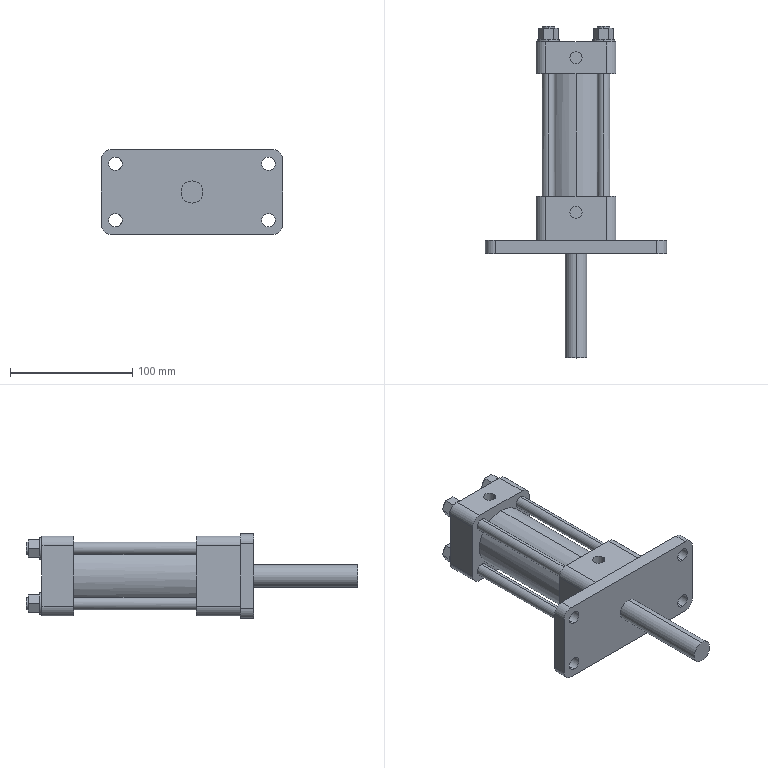Part | Creo | 1 solid | 108 faces | box 148 x 271 x 69 mm | volume 619155 mm3 | plane 56 | cylinder 52 | commonest cylinder face diameters 10 x20 16 x12 18 x10 11 x8 50 x2